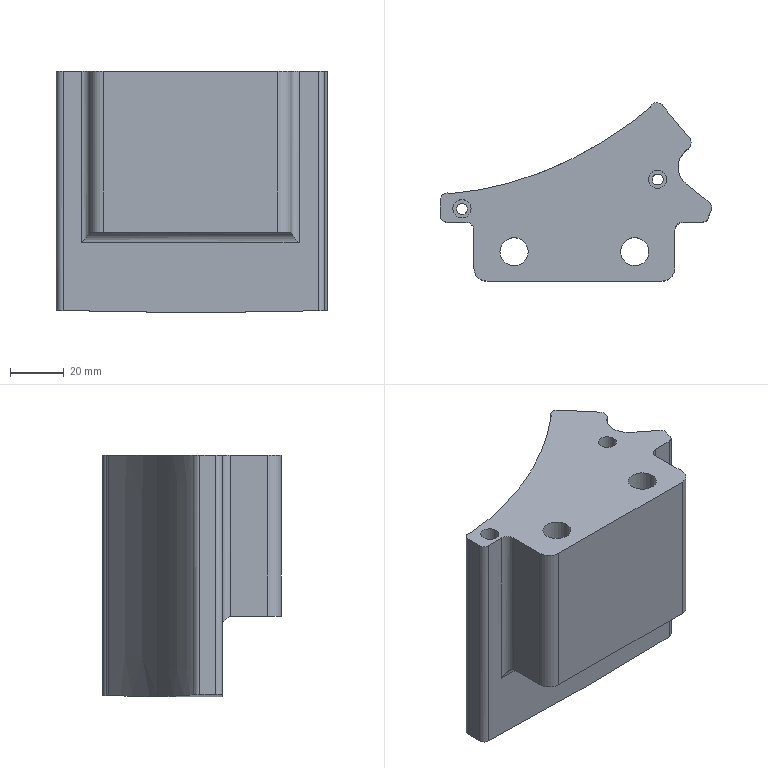Part | STEP file | gslz 2016.10.28-10_id3194_x_t | 1 solid | 43 faces | box 101.187 x 66.608 x 90 mm | volume 278822 mm3 | cylinder 23 | plane 18 | other 2 | commonest cylinder face diameters 5 x7 6 x3 4.1 x2 6.8 x2 10 x2 10.5 x2